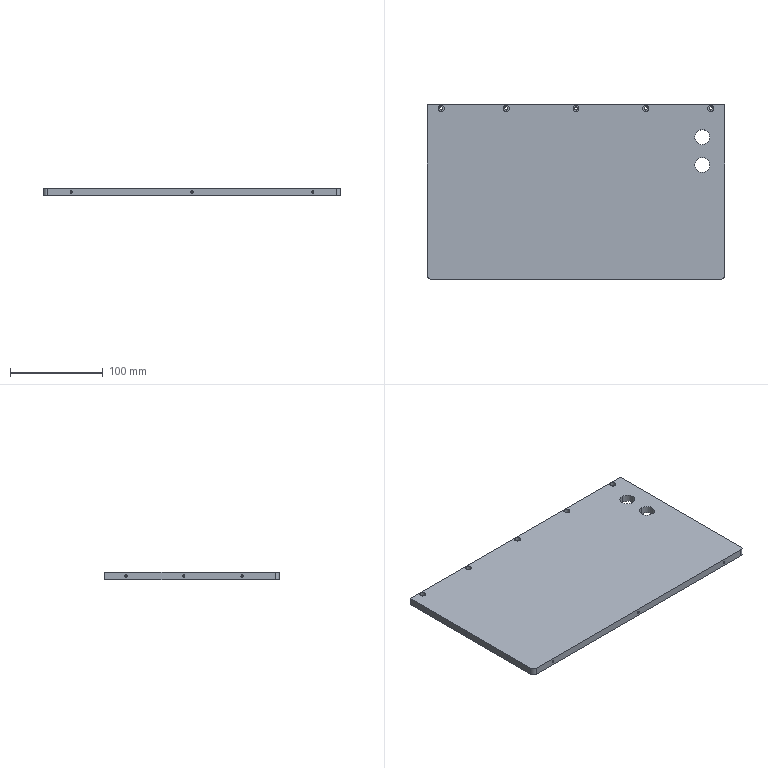NC program | Mastercam | posted with a generic post | part box 320 x 188 x 8 mm
Whole program:
%
O0000()
(MATERIAL - ALUMINUM MM - 2024)
( T1 | 10 FEM | H1 | XY STOCK TO LEAVE - .2 | Z STOCK TO LEAVE - 0. )
( T2 | 10 FEM | H2 | D2 | WEAR COMP | TOOL DIA. - 10. )
( T3 | 6 CHM | H3 )
N100 G21
N110 G0 G17 G40 G49 G80 G90
N120 T1 M6
N130 G0 G90 G54 X-149. Y-107.2 A0. S8000 M3
N140 G43 H1 Z60.
N150 Z1.
N160 G1 Z-8. F600.
N170 Y-105.2 F2000.
N180 G3 X-151. Y-103.2 I-2. J0.
N190 G1 X-156.
N200 G2 X-169.2 Y-90. I0. J13.2
N210 G1 Y-85.
N220 G3 X-171.2 Y-83. I-2. J0.
N230 G1 X-173.2
N240 X-171.2
N250 X-169.2
N260 G2 X-167.2 Y-85. I0. J-2.
N270 G1 Y-90.
N280 G3 X-156. Y-101.2 I11.2 J0.
N290 G1 X-151.
N300 G2 X-149. Y-103.2 I0. J-2.
N310 G1 Y-105.2
N320 Y-103.2
N330 Y-101.2
N340 G3 X-151. Y-99.2 I-2. J0.
N350 G1 X-156.
N360 G2 X-165.2 Y-90. I0. J9.2
N370 G1 Y-85.
N380 G3 X-167.2 Y-83. I-2. J0.
N390 G1 X-169.2
N400 G0 Z60.
N410 X173.2
N420 Z1.
N430 G1 Z-8. F600.
N440 X171.2 F2000.
N450 G3 X169.2 Y-85. I0. J-2.
N460 G1 Y-90.
N470 G2 X156. Y-103.2 I-13.2 J0.
N480 G1 X151.
N490 G3 X149. Y-105.2 I0. J-2.
N500 G1 Y-107.2
N510 Y-105.2
N520 Y-103.2
N530 G2 X151. Y-101.2 I2. J0.
N540 G1 X156.
N550 G3 X167.2 Y-90. I0. J11.2
N560 G1 Y-85.
N570 G2 X169.2 Y-83. I2. J0.
N580 G1 X171.2
N590 X169.2
N600 X167.2
N610 G3 X165.2 Y-85. I0. J-2.
N620 G1 Y-90.
N630 G2 X156. Y-99.2 I-9.2 J0.
N640 G1 X151.
N650 G3 X149. Y-101.2 I0. J-2.
N660 G1 Y-103.2
N670 G0 Z60.
N680 X-149. Y-105.2
N690 Z1.
N700 G1 Z-8. F600.
N710 Y-103.2 F2000.
N720 G3 X-151. Y-101.2 I-2. J0.
N730 G1 X-156.
N740 G2 X-167.2 Y-90. I0. J11.2
N750 G1 Y94.
N760 Y99.
N770 G3 X-169.2 Y101. I-2. J0.
N780 G1 X-171.2
N790 G0 Z60.
N800 X-149. Y-103.2
N810 Z1.
N820 G1 Z-8. F600.
N830 Y-101.2 F2000.
N840 G3 X-151. Y-99.2 I-2. J0.
N850 G1 X-156.
N860 G2 X-165.2 Y-90. I0. J9.2
N870 G1 Y94.
N880 Y99.
N890 G3 X-167.2 Y101. I-2. J0.
N900 G1 X-169.2
N910 G0 Z60.
N920 X171.2
N930 Z1.
N940 G1 Z-8. F600.
N950 X169.2 F2000.
N960 G3 X167.2 Y99. I0. J-2.
N970 G1 Y94.
N980 Y-90.
N990 G2 X156. Y-101.2 I-11.2 J0.
N1000 G1 X151.
N1010 G3 X149. Y-103.2 I0. J-2.
N1020 G1 Y-105.2
N1030 G0 Z60.
N1040 X169.2 Y101.
N1050 Z1.
N1060 G1 Z-8. F600.
N1070 X167.2 F2000.
N1080 G3 X165.2 Y99. I0. J-2.
N1090 G1 Y94.
N1100 Y-90.
N1110 G2 X156. Y-99.2 I-9.2 J0.
N1120 G1 X151.
N1130 G3 X149. Y-101.2 I0. J-2.
N1140 G1 Y-103.2
N1150 G0 Z60.
N1160 X136. Y56.2 Z20.
N1170 Z1.
N1180 G1 Z.3 F600.
N1190 G3 X138.8 Y59. Z.05 I0. J2.8 F3000.
N1200 X136. Y61.8 Z-.2 I-2.8 J0.
N1210 X133.2 Y59. Z-.45 I0. J-2.8
N1220 X136. Y56.2 Z-.7 I2.8 J0.
N1230 X138.8 Y59. Z-.95 I0. J2.8
N1240 X136. Y61.8 Z-1.2 I-2.8 J0.
N1250 X133.2 Y59. Z-1.45 I0. J-2.8
N1260 X136. Y56.2 Z-1.7 I2.8 J0.
N1270 X138.8 Y59. Z-1.95 I0. J2.8
N1280 X136. Y61.8 Z-2.2 I-2.8 J0.
N1290 X133.2 Y59. Z-2.45 I0. J-2.8
N1300 X136. Y56.2 Z-2.7 I2.8 J0.
N1310 X138.8 Y59. Z-2.95 I0. J2.8
N1320 X136. Y61.8 Z-3.2 I-2.8 J0.
N1330 X133.2 Y59. Z-3.45 I0. J-2.8
N1340 X136. Y56.2 Z-3.7 I2.8 J0.
N1350 X138.8 Y59. Z-3.95 I0. J2.8
N1360 X136. Y61.8 Z-4.2 I-2.8 J0.
N1370 X133.2 Y59. Z-4.45 I0. J-2.8
N1380 X136. Y56.2 Z-4.7 I2.8 J0.
N1390 X138.8 Y59. Z-4.95 I0. J2.8
N1400 X136. Y61.8 Z-5.2 I-2.8 J0.
N1410 X133.2 Y59. Z-5.45 I0. J-2.8
N1420 X136. Y56.2 Z-5.7 I2.8 J0.
N1430 X138.8 Y59. Z-5.95 I0. J2.8
N1440 X136. Y61.8 Z-6.2 I-2.8 J0.
N1450 X133.2 Y59. Z-6.45 I0. J-2.8
N1460 X136. Y56.2 Z-6.7 I2.8 J0.
N1470 X138.8 Y59. Z-6.95 I0. J2.8
N1480 X136. Y61.8 Z-7.2 I-2.8 J0.
N1490 X133.2 Y59. Z-7.45 I0. J-2.8
N1500 X136. Y56.2 Z-7.7 I2.8 J0.
N1510 X138.8 Y59. Z-7.95 I0. J2.8
N1520 X138.663 Y59.865 Z-8. I-2.8 J0.
N1530 X136. Y61.8 I-2.663 J-.865
N1540 X133.2 Y59. I0. J-2.8
N1550 X136. Y56.2 I2.8 J0.
N1560 X138.8 Y59. I0. J2.8
N1570 X138.663 Y59.865 I-2.8 J0.
N1580 G0 Z20.
N1590 X136. Y26.2
N1600 Z1.
N1610 G1 Z.3 F600.
N1620 G3 X138.8 Y29. Z.05 I0. J2.8 F3000.
N1630 X136. Y31.8 Z-.2 I-2.8 J0.
N1640 X133.2 Y29. Z-.45 I0. J-2.8
N1650 X136. Y26.2 Z-.7 I2.8 J0.
N1660 X138.8 Y29. Z-.95 I0. J2.8
N1670 X136. Y31.8 Z-1.2 I-2.8 J0.
N1680 X133.2 Y29. Z-1.45 I0. J-2.8
N1690 X136. Y26.2 Z-1.7 I2.8 J0.
N1700 X138.8 Y29. Z-1.95 I0. J2.8
N1710 X136. Y31.8 Z-2.2 I-2.8 J0.
N1720 X133.2 Y29. Z-2.45 I0. J-2.8
N1730 X136. Y26.2 Z-2.7 I2.8 J0.
N1740 X138.8 Y29. Z-2.95 I0. J2.8
N1750 X136. Y31.8 Z-3.2 I-2.8 J0.
N1760 X133.2 Y29. Z-3.45 I0. J-2.8
N1770 X136. Y26.2 Z-3.7 I2.8 J0.
N1780 X138.8 Y29. Z-3.95 I0. J2.8
N1790 X136. Y31.8 Z-4.2 I-2.8 J0.
N1800 X133.2 Y29. Z-4.45 I0. J-2.8
N1810 X136. Y26.2 Z-4.7 I2.8 J0.
N1820 X138.8 Y29. Z-4.95 I0. J2.8
N1830 X136. Y31.8 Z-5.2 I-2.8 J0.
N1840 X133.2 Y29. Z-5.45 I0. J-2.8
N1850 X136. Y26.2 Z-5.7 I2.8 J0.
N1860 X138.8 Y29. Z-5.95 I0. J2.8
N1870 X136. Y31.8 Z-6.2 I-2.8 J0.
N1880 X133.2 Y29. Z-6.45 I0. J-2.8
N1890 X136. Y26.2 Z-6.7 I2.8 J0.
N1900 X138.8 Y29. Z-6.95 I0. J2.8
N1910 X136. Y31.8 Z-7.2 I-2.8 J0.
N1920 X133.2 Y29. Z-7.45 I0. J-2.8
N1930 X136. Y26.2 Z-7.7 I2.8 J0.
N1940 X138.8 Y29. Z-7.95 I0. J2.8
N1950 X138.663 Y29.865 Z-8. I-2.8 J0.
N1960 X136. Y31.8 I-2.663 J-.865
N1970 X133.2 Y29. I0. J-2.8
N1980 X136. Y26.2 I2.8 J0.
N1990 X138.8 Y29. I0. J2.8
N2000 X138.663 Y29.865 I-2.8 J0.
N2010 G0 Z20.
N2020 M5
N2030 G91 G28 Z0.
N2040 A0.
N2050 M01
N2060 T2 M6
N2070 G0 G90 G17 G54 X-150.7 Y-99.6 A0. S8000 M3
N2080 G43 H2 Z60.
N2090 Z1.
N2100 G1 Z-8. F600.
N2110 G41 D2 Y-99.3 F1000.
N2120 G3 X-151. Y-99. I-.3 J0.
N2130 G1 X-156.
N2140 G2 X-165. Y-90. I0. J9.
N2150 G1 Y94.
N2160 Y99.
N2170 G3 X-165.3 Y99.3 I-.3 J0.
N2180 G1 G40 X-165.6
N2190 G0 Z60.
N2200 X165.6
N2210 Z1.
N2220 G1 Z-8. F600.
N2230 G41 D2 X165.3 F1000.
N2240 G3 X165. Y99. I0. J-.3
N2250 G1 Y94.
N2260 Y-90.
N2270 G2 X156. Y-99. I-9. J0.
N2280 G1 X151.
N2290 G3 X150.7 Y-99.3 I0. J-.3
N2300 G1 G40 Y-99.6
N2310 G0 Z60.
N2320 X136.3 Y61.4 Z20.
N2330 Z1.
N2340 G1 Z-8. F600.
N2350 G41 D2 Y61.7 F1000.
N2360 G3 X136. Y62. I-.3 J0.
N2370 X133. Y59. I0. J-3.
N2380 X136. Y56. I3. J0.
N2390 X139. Y59. I0. J3.
N2400 X136. Y62. I-3. J0.
N2410 X135.7 Y61.7 I0. J-.3
N2420 G1 G40 Y61.4
N2430 G0 Z20.
N2440 X136.3 Y31.4
N2450 Z1.
N2460 G1 Z-8. F600.
N2470 G41 D2 Y31.7 F1000.
N2480 G3 X136. Y32. I-.3 J0.
N2490 X133. Y29. I0. J-3.
N2500 X136. Y26. I3. J0.
N2510 X139. Y29. I0. J3.
N2520 X136. Y32. I-3. J0.
N2530 X135.7 Y31.7 I0. J-.3
N2540 G1 G40 Y31.4
N2550 G0 Z20.
N2560 M5
N2570 G91 G28 Z0.
N2580 A0.
N2590 M01
N2600 T3 M6
N2610 G0 G90 G17 G54 X-155.7 Y-95.75 A0. S5000 M3
N2620 G43 H3 Z60.
N2630 Z59.5
N2640 Z-.5
N2650 G1 Z-1.5 F600.
N2660 Y-95.45 F1000.
N2670 G3 X-156. Y-95.15 I-.3 J0.
N2680 G2 X-161.15 Y-90. I0. J5.15
N2690 G1 Y94.
N2700 G3 X-161.45 Y94.3 I-.3 J0.
N2710 G1 X-161.75
N2720 G0 Z58.5
N2730 Z60.
N2740 X135.7 Y52.75
N2750 Z59.5
N2760 Z-.5
N2770 G1 Z-1.5 F600.
N2780 Y52.45 F1000.
N2790 G3 X136. Y52.15 I.3 J0.
N2800 X142.85 Y59. I0. J6.85
N2810 X136. Y65.85 I-6.85 J0.
N2820 X129.15 Y59. I0. J-6.85
N2830 X136. Y52.15 I6.85 J0.
N2840 X136.3 Y52.45 I0. J.3
N2850 G1 Y52.75
N2860 G0 Z58.5
N2870 Z60.
N2880 X135.7 Y22.75
N2890 Z59.5
N2900 Z-.5
N2910 G1 Z-1.5 F600.
N2920 Y22.45 F1000.
N2930 G3 X136. Y22.15 I.3 J0.
N2940 X142.85 Y29. I0. J6.85
N2950 X136. Y35.85 I-6.85 J0.
N2960 X129.15 Y29. I0. J-6.85
N2970 X136. Y22.15 I6.85 J0.
N2980 X136.3 Y22.45 I0. J.3
N2990 G1 Y22.75
N3000 G0 Z58.5
N3010 Z60.
N3020 X149.025 Y58.525
N3030 X161.75 Y94.3
N3040 Z59.5
N3050 Z-.5
N3060 G1 Z-1.5 F600.
N3070 X161.45 F1000.
N3080 G3 X161.15 Y94. I0. J-.3
N3090 G1 Y-90.
N3100 G2 X156. Y-95.15 I-5.15 J0.
N3110 G3 X155.7 Y-95.45 I0. J-.3
N3120 G1 Y-95.75
N3130 G0 Z58.5
N3140 Z60.
N3150 M5
N3160 G91 G28 Z0.
N3170 G28 X0. Y0. A0.
N3180 M30
%